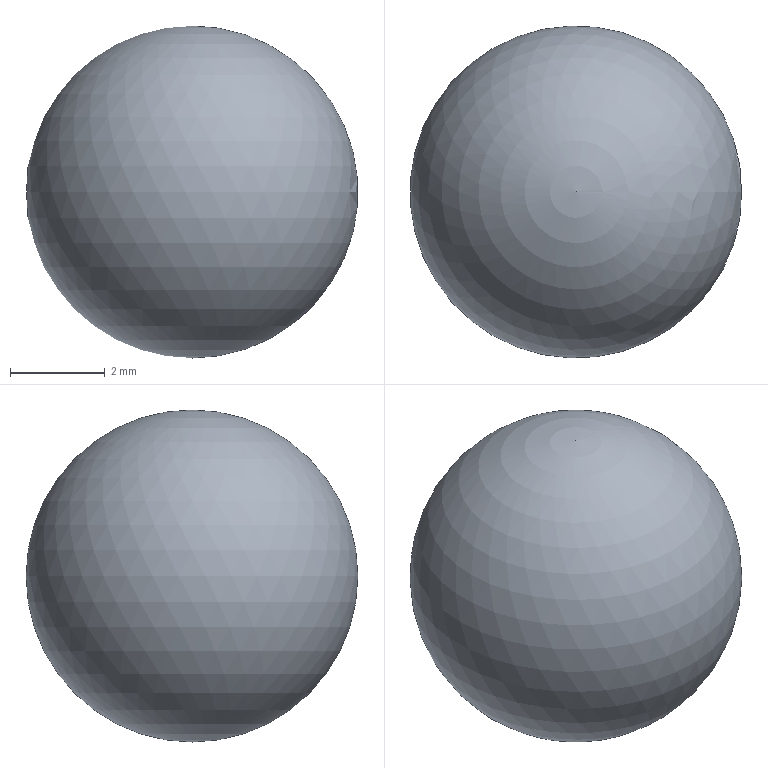Part | STEP file | 1-46.6 | 1 solid | 1 faces | box 7 x 7 x 7 mm | volume 179.594 mm3 | sphere 1
STEP:
#1=CARTESIAN_POINT('',(0.,0.,0.));
#2=DIRECTION('',(0.,0.,1.));
#3=DIRECTION('',(1.,0.,0.));
#4=AXIS2_PLACEMENT_3D('',#1,#2,#3);
#5=CARTESIAN_POINT('',(0.,0.,3.5));
#6=VERTEX_POINT('',#5);
#7=VERTEX_LOOP('',#6);
#8=FACE_BOUND('',#7,.T.);
#9=CARTESIAN_POINT('',(0.,0.,0.));
#10=DIRECTION('',(0.,0.,1.));
#11=DIRECTION('',(1.,0.,0.));
#12=AXIS2_PLACEMENT_3D('',#9,#10,#11);
#13=SPHERICAL_SURFACE('',#12,3.5);
#14=ADVANCED_FACE('',(#8),#13,.T.);
#15=CLOSED_SHELL('',(#14));
#16=MANIFOLD_SOLID_BREP('',#15);
#17=(LENGTH_UNIT()NAMED_UNIT(*)SI_UNIT(.MILLI.,.METRE.));
#18=UNCERTAINTY_MEASURE_WITH_UNIT(LENGTH_MEASURE(0.0000001),#17,'','');
#19=(NAMED_UNIT(*)PLANE_ANGLE_UNIT()SI_UNIT($,.RADIAN.));
#20=(NAMED_UNIT(*)SI_UNIT($,.STERADIAN.)SOLID_ANGLE_UNIT());
#21=(GEOMETRIC_REPRESENTATION_CONTEXT(3)GLOBAL_UNCERTAINTY_ASSIGNED_CONTEXT((#18))GLOBAL_UNIT_ASSIGNED_CONTEXT((#17,#19,#20))REPRESENTATION_CONTEXT('',''));
#22=ADVANCED_BREP_SHAPE_REPRESENTATION('',(#4,#16),#21);